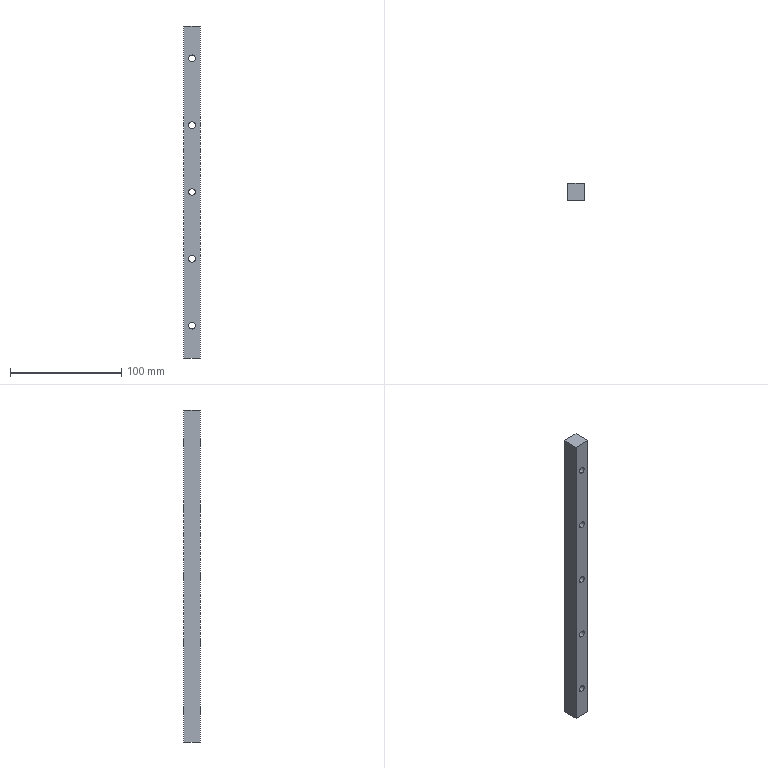Part | 1 solid | 16 faces | box 15 x 15 x 298 mm | volume 64929 mm3 | cylinder 10 | plane 6 | commonest cylinder face diameters 6 x10
STEP:
#1=CARTESIAN_POINT('',(7.5,0.,237.));
#2=VERTEX_POINT('',#1);
#3=CARTESIAN_POINT('',(7.5,0.,243.));
#4=VERTEX_POINT('',#3);
#5=CARTESIAN_POINT('',(7.5,0.,240.));
#6=DIRECTION('',(0.,1.,0.));
#7=DIRECTION('',(0.,0.,1.));
#8=AXIS2_PLACEMENT_3D('',#5,#6,#7);
#9=CIRCLE('',#8,3.);
#10=EDGE_CURVE('',#2,#4,#9,.T.);
#11=ORIENTED_EDGE('',*,*,#10,.F.);
#12=CARTESIAN_POINT('',(7.5,15.,237.));
#13=VERTEX_POINT('',#12);
#14=CARTESIAN_POINT('',(7.5,15.,237.));
#15=DIRECTION('',(0.,1.,0.));
#16=VECTOR('',#15,1000.);
#17=LINE('',#14,#16);
#18=EDGE_CURVE('',#2,#13,#17,.T.);
#19=ORIENTED_EDGE('',*,*,#18,.T.);
#20=CARTESIAN_POINT('',(7.5,15.,243.));
#21=VERTEX_POINT('',#20);
#22=CARTESIAN_POINT('',(7.5,15.,240.));
#23=DIRECTION('',(0.,1.,0.));
#24=DIRECTION('',(0.,0.,1.));
#25=AXIS2_PLACEMENT_3D('',#22,#23,#24);
#26=CIRCLE('',#25,3.);
#27=EDGE_CURVE('',#13,#21,#26,.T.);
#28=ORIENTED_EDGE('',*,*,#27,.T.);
#29=CARTESIAN_POINT('',(7.5,15.,243.));
#30=DIRECTION('',(0.,1.,0.));
#31=VECTOR('',#30,1000.);
#32=LINE('',#29,#31);
#33=EDGE_CURVE('',#4,#21,#32,.T.);
#34=ORIENTED_EDGE('',*,*,#33,.F.);
#35=EDGE_LOOP('',(#11,#19,#28,#34));
#36=FACE_OUTER_BOUND('',#35,.T.);
#37=CARTESIAN_POINT('',(7.5,15.,240.));
#38=DIRECTION('',(0.,1.,0.));
#39=DIRECTION('',(0.,0.,1.));
#40=AXIS2_PLACEMENT_3D('',#37,#38,#39);
#41=CYLINDRICAL_SURFACE('',#40,3.);
#42=ADVANCED_FACE('',(#36),#41,.F.);
#43=CARTESIAN_POINT('',(7.5,0.,297.));
#44=VERTEX_POINT('',#43);
#45=CARTESIAN_POINT('',(7.5,0.,303.));
#46=VERTEX_POINT('',#45);
#47=CARTESIAN_POINT('',(7.5,0.,300.));
#48=DIRECTION('',(0.,1.,0.));
#49=DIRECTION('',(0.,0.,1.));
#50=AXIS2_PLACEMENT_3D('',#47,#48,#49);
#51=CIRCLE('',#50,3.);
#52=EDGE_CURVE('',#44,#46,#51,.T.);
#53=ORIENTED_EDGE('',*,*,#52,.F.);
#54=CARTESIAN_POINT('',(7.5,15.,297.));
#55=VERTEX_POINT('',#54);
#56=CARTESIAN_POINT('',(7.5,15.,297.));
#57=DIRECTION('',(0.,1.,0.));
#58=VECTOR('',#57,1000.);
#59=LINE('',#56,#58);
#60=EDGE_CURVE('',#44,#55,#59,.T.);
#61=ORIENTED_EDGE('',*,*,#60,.T.);
#62=CARTESIAN_POINT('',(7.5,15.,303.));
#63=VERTEX_POINT('',#62);
#64=CARTESIAN_POINT('',(7.5,15.,300.));
#65=DIRECTION('',(0.,1.,0.));
#66=DIRECTION('',(0.,0.,1.));
#67=AXIS2_PLACEMENT_3D('',#64,#65,#66);
#68=CIRCLE('',#67,3.);
#69=EDGE_CURVE('',#55,#63,#68,.T.);
#70=ORIENTED_EDGE('',*,*,#69,.T.);
#71=CARTESIAN_POINT('',(7.5,15.,303.));
#72=DIRECTION('',(0.,1.,0.));
#73=VECTOR('',#72,1000.);
#74=LINE('',#71,#73);
#75=EDGE_CURVE('',#46,#63,#74,.T.);
#76=ORIENTED_EDGE('',*,*,#75,.F.);
#77=EDGE_LOOP('',(#53,#61,#70,#76));
#78=FACE_OUTER_BOUND('',#77,.T.);
#79=CARTESIAN_POINT('',(7.5,15.,300.));
#80=DIRECTION('',(0.,1.,0.));
#81=DIRECTION('',(0.,0.,1.));
#82=AXIS2_PLACEMENT_3D('',#79,#80,#81);
#83=CYLINDRICAL_SURFACE('',#82,3.);
#84=ADVANCED_FACE('',(#78),#83,.F.);
#85=CARTESIAN_POINT('',(7.5,0.,357.));
#86=VERTEX_POINT('',#85);
#87=CARTESIAN_POINT('',(7.5,0.,363.));
#88=VERTEX_POINT('',#87);
#89=CARTESIAN_POINT('',(7.5,0.,360.));
#90=DIRECTION('',(0.,1.,0.));
#91=DIRECTION('',(0.,0.,1.));
#92=AXIS2_PLACEMENT_3D('',#89,#90,#91);
#93=CIRCLE('',#92,3.);
#94=EDGE_CURVE('',#86,#88,#93,.T.);
#95=ORIENTED_EDGE('',*,*,#94,.F.);
#96=CARTESIAN_POINT('',(7.5,15.,357.));
#97=VERTEX_POINT('',#96);
#98=CARTESIAN_POINT('',(7.5,15.,357.));
#99=DIRECTION('',(0.,1.,0.));
#100=VECTOR('',#99,1000.);
#101=LINE('',#98,#100);
#102=EDGE_CURVE('',#86,#97,#101,.T.);
#103=ORIENTED_EDGE('',*,*,#102,.T.);
#104=CARTESIAN_POINT('',(7.5,15.,363.));
#105=VERTEX_POINT('',#104);
#106=CARTESIAN_POINT('',(7.5,15.,360.));
#107=DIRECTION('',(0.,1.,0.));
#108=DIRECTION('',(0.,0.,1.));
#109=AXIS2_PLACEMENT_3D('',#106,#107,#108);
#110=CIRCLE('',#109,3.);
#111=EDGE_CURVE('',#97,#105,#110,.T.);
#112=ORIENTED_EDGE('',*,*,#111,.T.);
#113=CARTESIAN_POINT('',(7.5,15.,363.));
#114=DIRECTION('',(0.,1.,0.));
#115=VECTOR('',#114,1000.);
#116=LINE('',#113,#115);
#117=EDGE_CURVE('',#88,#105,#116,.T.);
#118=ORIENTED_EDGE('',*,*,#117,.F.);
#119=EDGE_LOOP('',(#95,#103,#112,#118));
#120=FACE_OUTER_BOUND('',#119,.T.);
#121=CARTESIAN_POINT('',(7.5,15.,360.));
#122=DIRECTION('',(0.,1.,0.));
#123=DIRECTION('',(0.,0.,1.));
#124=AXIS2_PLACEMENT_3D('',#121,#122,#123);
#125=CYLINDRICAL_SURFACE('',#124,3.);
#126=ADVANCED_FACE('',(#120),#125,.F.);
#127=CARTESIAN_POINT('',(7.5,0.,417.));
#128=VERTEX_POINT('',#127);
#129=CARTESIAN_POINT('',(7.5,0.,423.));
#130=VERTEX_POINT('',#129);
#131=CARTESIAN_POINT('',(7.5,0.,420.));
#132=DIRECTION('',(0.,1.,0.));
#133=DIRECTION('',(0.,0.,1.));
#134=AXIS2_PLACEMENT_3D('',#131,#132,#133);
#135=CIRCLE('',#134,3.);
#136=EDGE_CURVE('',#128,#130,#135,.T.);
#137=ORIENTED_EDGE('',*,*,#136,.F.);
#138=CARTESIAN_POINT('',(7.5,15.,417.));
#139=VERTEX_POINT('',#138);
#140=CARTESIAN_POINT('',(7.5,15.,417.));
#141=DIRECTION('',(0.,1.,0.));
#142=VECTOR('',#141,1000.);
#143=LINE('',#140,#142);
#144=EDGE_CURVE('',#128,#139,#143,.T.);
#145=ORIENTED_EDGE('',*,*,#144,.T.);
#146=CARTESIAN_POINT('',(7.5,15.,423.));
#147=VERTEX_POINT('',#146);
#148=CARTESIAN_POINT('',(7.5,15.,420.));
#149=DIRECTION('',(0.,1.,0.));
#150=DIRECTION('',(0.,0.,1.));
#151=AXIS2_PLACEMENT_3D('',#148,#149,#150);
#152=CIRCLE('',#151,3.);
#153=EDGE_CURVE('',#139,#147,#152,.T.);
#154=ORIENTED_EDGE('',*,*,#153,.T.);
#155=CARTESIAN_POINT('',(7.5,15.,423.));
#156=DIRECTION('',(0.,1.,0.));
#157=VECTOR('',#156,1000.);
#158=LINE('',#155,#157);
#159=EDGE_CURVE('',#130,#147,#158,.T.);
#160=ORIENTED_EDGE('',*,*,#159,.F.);
#161=EDGE_LOOP('',(#137,#145,#154,#160));
#162=FACE_OUTER_BOUND('',#161,.T.);
#163=CARTESIAN_POINT('',(7.5,15.,420.));
#164=DIRECTION('',(0.,1.,0.));
#165=DIRECTION('',(0.,0.,1.));
#166=AXIS2_PLACEMENT_3D('',#163,#164,#165);
#167=CYLINDRICAL_SURFACE('',#166,3.);
#168=ADVANCED_FACE('',(#162),#167,.F.);
#169=CARTESIAN_POINT('',(7.5,0.,477.));
#170=VERTEX_POINT('',#169);
#171=CARTESIAN_POINT('',(7.5,0.,483.));
#172=VERTEX_POINT('',#171);
#173=CARTESIAN_POINT('',(7.5,0.,480.));
#174=DIRECTION('',(0.,1.,0.));
#175=DIRECTION('',(0.,0.,1.));
#176=AXIS2_PLACEMENT_3D('',#173,#174,#175);
#177=CIRCLE('',#176,3.);
#178=EDGE_CURVE('',#170,#172,#177,.T.);
#179=ORIENTED_EDGE('',*,*,#178,.F.);
#180=CARTESIAN_POINT('',(7.5,15.,477.));
#181=VERTEX_POINT('',#180);
#182=CARTESIAN_POINT('',(7.5,15.,477.));
#183=DIRECTION('',(0.,1.,0.));
#184=VECTOR('',#183,1000.);
#185=LINE('',#182,#184);
#186=EDGE_CURVE('',#170,#181,#185,.T.);
#187=ORIENTED_EDGE('',*,*,#186,.T.);
#188=CARTESIAN_POINT('',(7.5,15.,483.));
#189=VERTEX_POINT('',#188);
#190=CARTESIAN_POINT('',(7.5,15.,480.));
#191=DIRECTION('',(0.,1.,0.));
#192=DIRECTION('',(0.,0.,1.));
#193=AXIS2_PLACEMENT_3D('',#190,#191,#192);
#194=CIRCLE('',#193,3.);
#195=EDGE_CURVE('',#181,#189,#194,.T.);
#196=ORIENTED_EDGE('',*,*,#195,.T.);
#197=CARTESIAN_POINT('',(7.5,15.,483.));
#198=DIRECTION('',(0.,1.,0.));
#199=VECTOR('',#198,1000.);
#200=LINE('',#197,#199);
#201=EDGE_CURVE('',#172,#189,#200,.T.);
#202=ORIENTED_EDGE('',*,*,#201,.F.);
#203=EDGE_LOOP('',(#179,#187,#196,#202));
#204=FACE_OUTER_BOUND('',#203,.T.);
#205=CARTESIAN_POINT('',(7.5,15.,480.));
#206=DIRECTION('',(0.,1.,0.));
#207=DIRECTION('',(0.,0.,1.));
#208=AXIS2_PLACEMENT_3D('',#205,#206,#207);
#209=CYLINDRICAL_SURFACE('',#208,3.);
#210=ADVANCED_FACE('',(#204),#209,.F.);
#211=CARTESIAN_POINT('',(7.5,15.,240.));
#212=DIRECTION('',(0.,1.,0.));
#213=DIRECTION('',(0.,0.,1.));
#214=AXIS2_PLACEMENT_3D('',#211,#212,#213);
#215=CIRCLE('',#214,3.);
#216=EDGE_CURVE('',#21,#13,#215,.T.);
#217=ORIENTED_EDGE('',*,*,#216,.F.);
#218=ORIENTED_EDGE('',*,*,#27,.F.);
#219=EDGE_LOOP('',(#217,#218));
#220=FACE_BOUND('',#219,.T.);
#221=CARTESIAN_POINT('',(7.5,15.,300.));
#222=DIRECTION('',(0.,1.,0.));
#223=DIRECTION('',(0.,0.,1.));
#224=AXIS2_PLACEMENT_3D('',#221,#222,#223);
#225=CIRCLE('',#224,3.);
#226=EDGE_CURVE('',#63,#55,#225,.T.);
#227=ORIENTED_EDGE('',*,*,#226,.F.);
#228=ORIENTED_EDGE('',*,*,#69,.F.);
#229=EDGE_LOOP('',(#227,#228));
#230=FACE_BOUND('',#229,.T.);
#231=CARTESIAN_POINT('',(7.5,15.,360.));
#232=DIRECTION('',(0.,1.,0.));
#233=DIRECTION('',(0.,0.,1.));
#234=AXIS2_PLACEMENT_3D('',#231,#232,#233);
#235=CIRCLE('',#234,3.);
#236=EDGE_CURVE('',#105,#97,#235,.T.);
#237=ORIENTED_EDGE('',*,*,#236,.F.);
#238=ORIENTED_EDGE('',*,*,#111,.F.);
#239=EDGE_LOOP('',(#237,#238));
#240=FACE_BOUND('',#239,.T.);
#241=CARTESIAN_POINT('',(7.5,15.,420.));
#242=DIRECTION('',(0.,1.,0.));
#243=DIRECTION('',(0.,0.,1.));
#244=AXIS2_PLACEMENT_3D('',#241,#242,#243);
#245=CIRCLE('',#244,3.);
#246=EDGE_CURVE('',#147,#139,#245,.T.);
#247=ORIENTED_EDGE('',*,*,#246,.F.);
#248=ORIENTED_EDGE('',*,*,#153,.F.);
#249=EDGE_LOOP('',(#247,#248));
#250=FACE_BOUND('',#249,.T.);
#251=CARTESIAN_POINT('',(15.,15.,509.));
#252=VERTEX_POINT('',#251);
#253=CARTESIAN_POINT('',(15.,15.,211.));
#254=VERTEX_POINT('',#253);
#255=CARTESIAN_POINT('',(15.,15.,720.));
#256=DIRECTION('',(0.,0.,-1.));
#257=VECTOR('',#256,1000.);
#258=LINE('',#255,#257);
#259=EDGE_CURVE('',#252,#254,#258,.T.);
#260=ORIENTED_EDGE('',*,*,#259,.T.);
#261=CARTESIAN_POINT('',(0.,15.,211.));
#262=VERTEX_POINT('',#261);
#263=CARTESIAN_POINT('',(0.,15.,211.));
#264=DIRECTION('',(1.,0.,0.));
#265=VECTOR('',#264,1000.);
#266=LINE('',#263,#265);
#267=EDGE_CURVE('',#262,#254,#266,.T.);
#268=ORIENTED_EDGE('',*,*,#267,.F.);
#269=CARTESIAN_POINT('',(0.,15.,509.));
#270=VERTEX_POINT('',#269);
#271=CARTESIAN_POINT('',(0.,15.,720.));
#272=DIRECTION('',(0.,0.,-1.));
#273=VECTOR('',#272,1000.);
#274=LINE('',#271,#273);
#275=EDGE_CURVE('',#270,#262,#274,.T.);
#276=ORIENTED_EDGE('',*,*,#275,.F.);
#277=CARTESIAN_POINT('',(0.,15.,509.));
#278=DIRECTION('',(-1.,0.,0.));
#279=VECTOR('',#278,1000.);
#280=LINE('',#277,#279);
#281=EDGE_CURVE('',#252,#270,#280,.T.);
#282=ORIENTED_EDGE('',*,*,#281,.F.);
#283=EDGE_LOOP('',(#260,#268,#276,#282));
#284=FACE_OUTER_BOUND('',#283,.T.);
#285=CARTESIAN_POINT('',(7.5,15.,480.));
#286=DIRECTION('',(0.,1.,0.));
#287=DIRECTION('',(0.,0.,1.));
#288=AXIS2_PLACEMENT_3D('',#285,#286,#287);
#289=CIRCLE('',#288,3.);
#290=EDGE_CURVE('',#189,#181,#289,.T.);
#291=ORIENTED_EDGE('',*,*,#290,.F.);
#292=ORIENTED_EDGE('',*,*,#195,.F.);
#293=EDGE_LOOP('',(#291,#292));
#294=FACE_BOUND('',#293,.T.);
#295=CARTESIAN_POINT('',(0.,15.,720.));
#296=DIRECTION('',(0.,-1.,0.));
#297=DIRECTION('',(0.,0.,-1.));
#298=AXIS2_PLACEMENT_3D('',#295,#296,#297);
#299=PLANE('',#298);
#300=ADVANCED_FACE('',(#220,#230,#240,#250,#284,#294),#299,.F.);
#301=ORIENTED_EDGE('',*,*,#275,.T.);
#302=CARTESIAN_POINT('',(0.,0.,211.));
#303=VERTEX_POINT('',#302);
#304=CARTESIAN_POINT('',(0.,0.,211.));
#305=DIRECTION('',(0.,1.,0.));
#306=VECTOR('',#305,1000.);
#307=LINE('',#304,#306);
#308=EDGE_CURVE('',#303,#262,#307,.T.);
#309=ORIENTED_EDGE('',*,*,#308,.F.);
#310=CARTESIAN_POINT('',(0.,0.,509.));
#311=VERTEX_POINT('',#310);
#312=CARTESIAN_POINT('',(0.,0.,720.));
#313=DIRECTION('',(0.,0.,-1.));
#314=VECTOR('',#313,1000.);
#315=LINE('',#312,#314);
#316=EDGE_CURVE('',#311,#303,#315,.T.);
#317=ORIENTED_EDGE('',*,*,#316,.F.);
#318=CARTESIAN_POINT('',(0.,0.,509.));
#319=DIRECTION('',(0.,1.,0.));
#320=VECTOR('',#319,1000.);
#321=LINE('',#318,#320);
#322=EDGE_CURVE('',#311,#270,#321,.T.);
#323=ORIENTED_EDGE('',*,*,#322,.T.);
#324=EDGE_LOOP('',(#301,#309,#317,#323));
#325=FACE_OUTER_BOUND('',#324,.T.);
#326=CARTESIAN_POINT('',(0.,0.,720.));
#327=DIRECTION('',(1.,0.,0.));
#328=DIRECTION('',(0.,0.,-1.));
#329=AXIS2_PLACEMENT_3D('',#326,#327,#328);
#330=PLANE('',#329);
#331=ADVANCED_FACE('',(#325),#330,.F.);
#332=CARTESIAN_POINT('',(7.5,0.,240.));
#333=DIRECTION('',(0.,1.,0.));
#334=DIRECTION('',(0.,0.,1.));
#335=AXIS2_PLACEMENT_3D('',#332,#333,#334);
#336=CIRCLE('',#335,3.);
#337=EDGE_CURVE('',#4,#2,#336,.T.);
#338=ORIENTED_EDGE('',*,*,#337,.T.);
#339=ORIENTED_EDGE('',*,*,#10,.T.);
#340=EDGE_LOOP('',(#338,#339));
#341=FACE_BOUND('',#340,.T.);
#342=CARTESIAN_POINT('',(7.5,0.,300.));
#343=DIRECTION('',(0.,1.,0.));
#344=DIRECTION('',(0.,0.,1.));
#345=AXIS2_PLACEMENT_3D('',#342,#343,#344);
#346=CIRCLE('',#345,3.);
#347=EDGE_CURVE('',#46,#44,#346,.T.);
#348=ORIENTED_EDGE('',*,*,#347,.T.);
#349=ORIENTED_EDGE('',*,*,#52,.T.);
#350=EDGE_LOOP('',(#348,#349));
#351=FACE_BOUND('',#350,.T.);
#352=CARTESIAN_POINT('',(7.5,0.,360.));
#353=DIRECTION('',(0.,1.,0.));
#354=DIRECTION('',(0.,0.,1.));
#355=AXIS2_PLACEMENT_3D('',#352,#353,#354);
#356=CIRCLE('',#355,3.);
#357=EDGE_CURVE('',#88,#86,#356,.T.);
#358=ORIENTED_EDGE('',*,*,#357,.T.);
#359=ORIENTED_EDGE('',*,*,#94,.T.);
#360=EDGE_LOOP('',(#358,#359));
#361=FACE_BOUND('',#360,.T.);
#362=CARTESIAN_POINT('',(7.5,0.,420.));
#363=DIRECTION('',(0.,1.,0.));
#364=DIRECTION('',(0.,0.,1.));
#365=AXIS2_PLACEMENT_3D('',#362,#363,#364);
#366=CIRCLE('',#365,3.);
#367=EDGE_CURVE('',#130,#128,#366,.T.);
#368=ORIENTED_EDGE('',*,*,#367,.T.);
#369=ORIENTED_EDGE('',*,*,#136,.T.);
#370=EDGE_LOOP('',(#368,#369));
#371=FACE_BOUND('',#370,.T.);
#372=CARTESIAN_POINT('',(7.5,0.,480.));
#373=DIRECTION('',(0.,1.,0.));
#374=DIRECTION('',(0.,0.,1.));
#375=AXIS2_PLACEMENT_3D('',#372,#373,#374);
#376=CIRCLE('',#375,3.);
#377=EDGE_CURVE('',#172,#170,#376,.T.);
#378=ORIENTED_EDGE('',*,*,#377,.T.);
#379=ORIENTED_EDGE('',*,*,#178,.T.);
#380=EDGE_LOOP('',(#378,#379));
#381=FACE_BOUND('',#380,.T.);
#382=ORIENTED_EDGE('',*,*,#316,.T.);
#383=CARTESIAN_POINT('',(15.,0.,211.));
#384=VERTEX_POINT('',#383);
#385=CARTESIAN_POINT('',(0.,0.,211.));
#386=DIRECTION('',(1.,0.,0.));
#387=VECTOR('',#386,1000.);
#388=LINE('',#385,#387);
#389=EDGE_CURVE('',#303,#384,#388,.T.);
#390=ORIENTED_EDGE('',*,*,#389,.T.);
#391=CARTESIAN_POINT('',(15.,0.,509.));
#392=VERTEX_POINT('',#391);
#393=CARTESIAN_POINT('',(15.,0.,720.));
#394=DIRECTION('',(0.,0.,-1.));
#395=VECTOR('',#394,1000.);
#396=LINE('',#393,#395);
#397=EDGE_CURVE('',#392,#384,#396,.T.);
#398=ORIENTED_EDGE('',*,*,#397,.F.);
#399=CARTESIAN_POINT('',(0.,0.,509.));
#400=DIRECTION('',(-1.,0.,0.));
#401=VECTOR('',#400,1000.);
#402=LINE('',#399,#401);
#403=EDGE_CURVE('',#392,#311,#402,.T.);
#404=ORIENTED_EDGE('',*,*,#403,.T.);
#405=EDGE_LOOP('',(#382,#390,#398,#404));
#406=FACE_OUTER_BOUND('',#405,.T.);
#407=CARTESIAN_POINT('',(0.,0.,720.));
#408=DIRECTION('',(0.,1.,0.));
#409=DIRECTION('',(0.,0.,1.));
#410=AXIS2_PLACEMENT_3D('',#407,#408,#409);
#411=PLANE('',#410);
#412=ADVANCED_FACE('',(#341,#351,#361,#371,#381,#406),#411,.F.);
#413=ORIENTED_EDGE('',*,*,#397,.T.);
#414=CARTESIAN_POINT('',(15.,0.,211.));
#415=DIRECTION('',(0.,1.,0.));
#416=VECTOR('',#415,1000.);
#417=LINE('',#414,#416);
#418=EDGE_CURVE('',#384,#254,#417,.T.);
#419=ORIENTED_EDGE('',*,*,#418,.T.);
#420=ORIENTED_EDGE('',*,*,#259,.F.);
#421=CARTESIAN_POINT('',(15.,0.,509.));
#422=DIRECTION('',(0.,1.,0.));
#423=VECTOR('',#422,1000.);
#424=LINE('',#421,#423);
#425=EDGE_CURVE('',#392,#252,#424,.T.);
#426=ORIENTED_EDGE('',*,*,#425,.F.);
#427=EDGE_LOOP('',(#413,#419,#420,#426));
#428=FACE_OUTER_BOUND('',#427,.T.);
#429=CARTESIAN_POINT('',(15.,0.,720.));
#430=DIRECTION('',(-1.,0.,0.));
#431=DIRECTION('',(0.,0.,1.));
#432=AXIS2_PLACEMENT_3D('',#429,#430,#431);
#433=PLANE('',#432);
#434=ADVANCED_FACE('',(#428),#433,.F.);
#435=ORIENTED_EDGE('',*,*,#281,.T.);
#436=ORIENTED_EDGE('',*,*,#322,.F.);
#437=ORIENTED_EDGE('',*,*,#403,.F.);
#438=ORIENTED_EDGE('',*,*,#425,.T.);
#439=EDGE_LOOP('',(#435,#436,#437,#438));
#440=FACE_OUTER_BOUND('',#439,.T.);
#441=CARTESIAN_POINT('',(0.,0.,509.));
#442=DIRECTION('',(0.,0.,-1.));
#443=DIRECTION('',(-1.,0.,0.));
#444=AXIS2_PLACEMENT_3D('',#441,#442,#443);
#445=PLANE('',#444);
#446=ADVANCED_FACE('',(#440),#445,.F.);
#447=ORIENTED_EDGE('',*,*,#267,.T.);
#448=ORIENTED_EDGE('',*,*,#418,.F.);
#449=ORIENTED_EDGE('',*,*,#389,.F.);
#450=ORIENTED_EDGE('',*,*,#308,.T.);
#451=EDGE_LOOP('',(#447,#448,#449,#450));
#452=FACE_OUTER_BOUND('',#451,.T.);
#453=CARTESIAN_POINT('',(0.,0.,211.));
#454=DIRECTION('',(0.,0.,1.));
#455=DIRECTION('',(1.,0.,0.));
#456=AXIS2_PLACEMENT_3D('',#453,#454,#455);
#457=PLANE('',#456);
#458=ADVANCED_FACE('',(#452),#457,.F.);
#459=ORIENTED_EDGE('',*,*,#186,.F.);
#460=ORIENTED_EDGE('',*,*,#377,.F.);
#461=ORIENTED_EDGE('',*,*,#201,.T.);
#462=ORIENTED_EDGE('',*,*,#290,.T.);
#463=EDGE_LOOP('',(#459,#460,#461,#462));
#464=FACE_OUTER_BOUND('',#463,.T.);
#465=CARTESIAN_POINT('',(7.5,15.,480.));
#466=DIRECTION('',(0.,1.,0.));
#467=DIRECTION('',(0.,0.,1.));
#468=AXIS2_PLACEMENT_3D('',#465,#466,#467);
#469=CYLINDRICAL_SURFACE('',#468,3.);
#470=ADVANCED_FACE('',(#464),#469,.F.);
#471=ORIENTED_EDGE('',*,*,#144,.F.);
#472=ORIENTED_EDGE('',*,*,#367,.F.);
#473=ORIENTED_EDGE('',*,*,#159,.T.);
#474=ORIENTED_EDGE('',*,*,#246,.T.);
#475=EDGE_LOOP('',(#471,#472,#473,#474));
#476=FACE_OUTER_BOUND('',#475,.T.);
#477=CARTESIAN_POINT('',(7.5,15.,420.));
#478=DIRECTION('',(0.,1.,0.));
#479=DIRECTION('',(0.,0.,1.));
#480=AXIS2_PLACEMENT_3D('',#477,#478,#479);
#481=CYLINDRICAL_SURFACE('',#480,3.);
#482=ADVANCED_FACE('',(#476),#481,.F.);
#483=ORIENTED_EDGE('',*,*,#102,.F.);
#484=ORIENTED_EDGE('',*,*,#357,.F.);
#485=ORIENTED_EDGE('',*,*,#117,.T.);
#486=ORIENTED_EDGE('',*,*,#236,.T.);
#487=EDGE_LOOP('',(#483,#484,#485,#486));
#488=FACE_OUTER_BOUND('',#487,.T.);
#489=CARTESIAN_POINT('',(7.5,15.,360.));
#490=DIRECTION('',(0.,1.,0.));
#491=DIRECTION('',(0.,0.,1.));
#492=AXIS2_PLACEMENT_3D('',#489,#490,#491);
#493=CYLINDRICAL_SURFACE('',#492,3.);
#494=ADVANCED_FACE('',(#488),#493,.F.);
#495=ORIENTED_EDGE('',*,*,#60,.F.);
#496=ORIENTED_EDGE('',*,*,#347,.F.);
#497=ORIENTED_EDGE('',*,*,#75,.T.);
#498=ORIENTED_EDGE('',*,*,#226,.T.);
#499=EDGE_LOOP('',(#495,#496,#497,#498));
#500=FACE_OUTER_BOUND('',#499,.T.);
#501=CARTESIAN_POINT('',(7.5,15.,300.));
#502=DIRECTION('',(0.,1.,0.));
#503=DIRECTION('',(0.,0.,1.));
#504=AXIS2_PLACEMENT_3D('',#501,#502,#503);
#505=CYLINDRICAL_SURFACE('',#504,3.);
#506=ADVANCED_FACE('',(#500),#505,.F.);
#507=ORIENTED_EDGE('',*,*,#18,.F.);
#508=ORIENTED_EDGE('',*,*,#337,.F.);
#509=ORIENTED_EDGE('',*,*,#33,.T.);
#510=ORIENTED_EDGE('',*,*,#216,.T.);
#511=EDGE_LOOP('',(#507,#508,#509,#510));
#512=FACE_OUTER_BOUND('',#511,.T.);
#513=CARTESIAN_POINT('',(7.5,15.,240.));
#514=DIRECTION('',(0.,1.,0.));
#515=DIRECTION('',(0.,0.,1.));
#516=AXIS2_PLACEMENT_3D('',#513,#514,#515);
#517=CYLINDRICAL_SURFACE('',#516,3.);
#518=ADVANCED_FACE('',(#512),#517,.F.);
#519=CLOSED_SHELL('',(#42,#84,#126,#168,#210,#300,#331,#412,#434,#446,#458,#470,#482,#494,#506,#518));
#520=MANIFOLD_SOLID_BREP('',#519);
#521=CARTESIAN_POINT('',(0.,0.,0.));
#522=DIRECTION('',(0.,0.,1.));
#523=DIRECTION('',(1.,0.,0.));
#524=AXIS2_PLACEMENT_3D('',#521,#522,#523);
#525=(LENGTH_UNIT()NAMED_UNIT(*)SI_UNIT(.MILLI.,.METRE.));
#526=UNCERTAINTY_MEASURE_WITH_UNIT(LENGTH_MEASURE(0.00001),#525,'','');
#527=(NAMED_UNIT(*)PLANE_ANGLE_UNIT()SI_UNIT($,.RADIAN.));
#528=(NAMED_UNIT(*)SI_UNIT($,.STERADIAN.)SOLID_ANGLE_UNIT());
#529=(GEOMETRIC_REPRESENTATION_CONTEXT(3)GLOBAL_UNCERTAINTY_ASSIGNED_CONTEXT((#526))GLOBAL_UNIT_ASSIGNED_CONTEXT((#525,#527,#528))REPRESENTATION_CONTEXT('',''));
#530=ADVANCED_BREP_SHAPE_REPRESENTATION('',(#520,#524),#529);